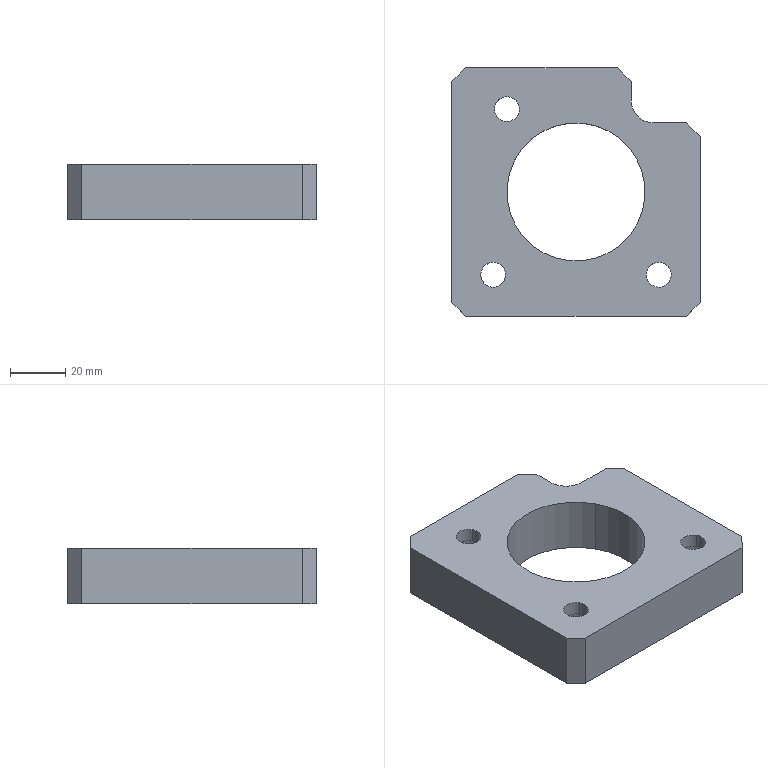Part | CATIA | 1 solid | 31 faces | box 90 x 90 x 20 mm | volume 102848 mm3 | plane 16 | cylinder 15 | commonest cylinder face diameters 9 x6 15 x6 50 x2 16 x1
STEP:
#1=CARTESIAN_POINT('',(500.,-120.,-5.5));
#2=VERTEX_POINT('',#1);
#3=CARTESIAN_POINT('',(500.,-120.,14.5));
#4=VERTEX_POINT('',#3);
#5=CARTESIAN_POINT('',(500.,-120.,4.5));
#6=DIRECTION('',(0.,0.,-1.));
#7=VECTOR('',#6,1.);
#8=LINE('',#5,#7);
#9=EDGE_CURVE('',#2,#4,#8,.F.);
#10=ORIENTED_EDGE('',*,*,#9,.F.);
#11=CARTESIAN_POINT('',(495.,-125.,-5.5));
#12=VERTEX_POINT('',#11);
#13=CARTESIAN_POINT('',(497.5,-122.5,-5.5));
#14=DIRECTION('',(0.7071,0.7071,0.));
#15=VECTOR('',#14,1.);
#16=LINE('',#13,#15);
#17=EDGE_CURVE('',#2,#12,#16,.F.);
#18=ORIENTED_EDGE('',*,*,#17,.T.);
#19=CARTESIAN_POINT('',(495.,-125.,14.5));
#20=VERTEX_POINT('',#19);
#21=CARTESIAN_POINT('',(495.,-125.,4.5));
#22=DIRECTION('',(0.,0.,-1.));
#23=VECTOR('',#22,1.);
#24=LINE('',#21,#23);
#25=EDGE_CURVE('',#12,#20,#24,.F.);
#26=ORIENTED_EDGE('',*,*,#25,.T.);
#27=CARTESIAN_POINT('',(497.5,-122.5,14.5));
#28=DIRECTION('',(0.7071,0.7071,0.));
#29=VECTOR('',#28,1.);
#30=LINE('',#27,#29);
#31=EDGE_CURVE('',#20,#4,#30,.T.);
#32=ORIENTED_EDGE('',*,*,#31,.T.);
#33=EDGE_LOOP('',(#10,#18,#26,#32));
#34=FACE_OUTER_BOUND('',#33,.T.);
#35=CARTESIAN_POINT('',(495.,-125.,18.5));
#36=DIRECTION('',(0.7071,-0.7071,0.));
#37=DIRECTION('',(0.,0.,-1.));
#38=AXIS2_PLACEMENT_3D('',#35,#36,#37);
#39=PLANE('',#38);
#40=ADVANCED_FACE('',(#34),#39,.F.);
#41=CARTESIAN_POINT('',(495.,-205.,-5.5));
#42=VERTEX_POINT('',#41);
#43=CARTESIAN_POINT('',(495.,-205.,14.5));
#44=VERTEX_POINT('',#43);
#45=CARTESIAN_POINT('',(495.,-205.,4.5));
#46=DIRECTION('',(0.,0.,1.));
#47=VECTOR('',#46,1.);
#48=LINE('',#45,#47);
#49=EDGE_CURVE('',#42,#44,#48,.T.);
#50=ORIENTED_EDGE('',*,*,#49,.T.);
#51=CARTESIAN_POINT('',(495.,-165.,14.5));
#52=DIRECTION('',(0.,1.,0.));
#53=VECTOR('',#52,1.);
#54=LINE('',#51,#53);
#55=EDGE_CURVE('',#20,#44,#54,.F.);
#56=ORIENTED_EDGE('',*,*,#55,.F.);
#57=ORIENTED_EDGE('',*,*,#25,.F.);
#58=CARTESIAN_POINT('',(495.,-165.,-5.5));
#59=DIRECTION('',(0.,1.,0.));
#60=VECTOR('',#59,1.);
#61=LINE('',#58,#60);
#62=EDGE_CURVE('',#12,#42,#61,.F.);
#63=ORIENTED_EDGE('',*,*,#62,.T.);
#64=EDGE_LOOP('',(#50,#56,#57,#63));
#65=FACE_OUTER_BOUND('',#64,.T.);
#66=CARTESIAN_POINT('',(495.,-210.,-5.5));
#67=DIRECTION('',(1.,0.,0.));
#68=DIRECTION('',(0.,1.,0.));
#69=AXIS2_PLACEMENT_3D('',#66,#67,#68);
#70=PLANE('',#69);
#71=ADVANCED_FACE('',(#65),#70,.F.);
#72=ORIENTED_EDGE('',*,*,#49,.F.);
#73=CARTESIAN_POINT('',(500.,-210.,-5.5));
#74=VERTEX_POINT('',#73);
#75=CARTESIAN_POINT('',(497.5,-207.5,-5.5));
#76=DIRECTION('',(0.7071,-0.7071,0.));
#77=VECTOR('',#76,1.);
#78=LINE('',#75,#77);
#79=EDGE_CURVE('',#42,#74,#78,.T.);
#80=ORIENTED_EDGE('',*,*,#79,.T.);
#81=CARTESIAN_POINT('',(500.,-210.,14.5));
#82=VERTEX_POINT('',#81);
#83=CARTESIAN_POINT('',(500.,-210.,4.5));
#84=DIRECTION('',(0.,0.,1.));
#85=VECTOR('',#84,1.);
#86=LINE('',#83,#85);
#87=EDGE_CURVE('',#74,#82,#86,.T.);
#88=ORIENTED_EDGE('',*,*,#87,.T.);
#89=CARTESIAN_POINT('',(497.5,-207.5,14.5));
#90=DIRECTION('',(0.7071,-0.7071,0.));
#91=VECTOR('',#90,1.);
#92=LINE('',#89,#91);
#93=EDGE_CURVE('',#82,#44,#92,.F.);
#94=ORIENTED_EDGE('',*,*,#93,.T.);
#95=EDGE_LOOP('',(#72,#80,#88,#94));
#96=FACE_OUTER_BOUND('',#95,.T.);
#97=CARTESIAN_POINT('',(495.,-205.,-9.5));
#98=DIRECTION('',(0.7071,0.7071,0.));
#99=DIRECTION('',(0.,0.,1.));
#100=AXIS2_PLACEMENT_3D('',#97,#98,#99);
#101=PLANE('',#100);
#102=ADVANCED_FACE('',(#96),#101,.F.);
#103=CARTESIAN_POINT('',(580.,-210.,-5.5));
#104=VERTEX_POINT('',#103);
#105=CARTESIAN_POINT('',(580.,-210.,14.5));
#106=VERTEX_POINT('',#105);
#107=CARTESIAN_POINT('',(580.,-210.,4.5));
#108=DIRECTION('',(0.,0.,-1.));
#109=VECTOR('',#108,1.);
#110=LINE('',#107,#109);
#111=EDGE_CURVE('',#104,#106,#110,.F.);
#112=ORIENTED_EDGE('',*,*,#111,.T.);
#113=CARTESIAN_POINT('',(540.,-210.,14.5));
#114=DIRECTION('',(-1.,0.,0.));
#115=VECTOR('',#114,1.);
#116=LINE('',#113,#115);
#117=EDGE_CURVE('',#82,#106,#116,.F.);
#118=ORIENTED_EDGE('',*,*,#117,.F.);
#119=ORIENTED_EDGE('',*,*,#87,.F.);
#120=CARTESIAN_POINT('',(540.,-210.,-5.5));
#121=DIRECTION('',(-1.,0.,0.));
#122=VECTOR('',#121,1.);
#123=LINE('',#120,#122);
#124=EDGE_CURVE('',#74,#104,#123,.F.);
#125=ORIENTED_EDGE('',*,*,#124,.T.);
#126=EDGE_LOOP('',(#112,#118,#119,#125));
#127=FACE_OUTER_BOUND('',#126,.T.);
#128=CARTESIAN_POINT('',(585.,-210.,-5.5));
#129=DIRECTION('',(0.,1.,0.));
#130=DIRECTION('',(-1.,0.,0.));
#131=AXIS2_PLACEMENT_3D('',#128,#129,#130);
#132=PLANE('',#131);
#133=ADVANCED_FACE('',(#127),#132,.F.);
#134=ORIENTED_EDGE('',*,*,#111,.F.);
#135=CARTESIAN_POINT('',(585.,-205.,-5.5));
#136=VERTEX_POINT('',#135);
#137=CARTESIAN_POINT('',(582.5,-207.5,-5.5));
#138=DIRECTION('',(-0.7071,-0.7071,0.));
#139=VECTOR('',#138,1.);
#140=LINE('',#137,#139);
#141=EDGE_CURVE('',#104,#136,#140,.F.);
#142=ORIENTED_EDGE('',*,*,#141,.T.);
#143=CARTESIAN_POINT('',(585.,-205.,14.5));
#144=VERTEX_POINT('',#143);
#145=CARTESIAN_POINT('',(585.,-205.,4.5));
#146=DIRECTION('',(0.,0.,-1.));
#147=VECTOR('',#146,1.);
#148=LINE('',#145,#147);
#149=EDGE_CURVE('',#136,#144,#148,.F.);
#150=ORIENTED_EDGE('',*,*,#149,.T.);
#151=CARTESIAN_POINT('',(582.5,-207.5,14.5));
#152=DIRECTION('',(-0.7071,-0.7071,0.));
#153=VECTOR('',#152,1.);
#154=LINE('',#151,#153);
#155=EDGE_CURVE('',#144,#106,#154,.T.);
#156=ORIENTED_EDGE('',*,*,#155,.T.);
#157=EDGE_LOOP('',(#134,#142,#150,#156));
#158=FACE_OUTER_BOUND('',#157,.T.);
#159=CARTESIAN_POINT('',(585.,-205.,18.5));
#160=DIRECTION('',(-0.7071,0.7071,0.));
#161=DIRECTION('',(0.,0.,-1.));
#162=AXIS2_PLACEMENT_3D('',#159,#160,#161);
#163=PLANE('',#162);
#164=ADVANCED_FACE('',(#158),#163,.F.);
#165=CARTESIAN_POINT('',(518.06,-176.986,14.5));
#166=VERTEX_POINT('',#165);
#167=CARTESIAN_POINT('',(561.94,-153.014,14.5));
#168=VERTEX_POINT('',#167);
#169=CARTESIAN_POINT('',(540.,-165.,14.5));
#170=DIRECTION('',(0.,0.,1.));
#171=AXIS2_PLACEMENT_3D('',#169,#170,$);
#172=CIRCLE('',#171,25.);
#173=EDGE_CURVE('',#166,#168,#172,.T.);
#174=ORIENTED_EDGE('',*,*,#173,.T.);
#175=CARTESIAN_POINT('',(561.94,-153.014,-5.5));
#176=VERTEX_POINT('',#175);
#177=CARTESIAN_POINT('',(561.94,-153.014,9.3));
#178=DIRECTION('',(0.,0.,1.));
#179=VECTOR('',#178,1.);
#180=LINE('',#177,#179);
#181=EDGE_CURVE('',#168,#176,#180,.F.);
#182=ORIENTED_EDGE('',*,*,#181,.T.);
#183=CARTESIAN_POINT('',(518.06,-176.986,-5.5));
#184=VERTEX_POINT('',#183);
#185=CARTESIAN_POINT('',(540.,-165.,-5.5));
#186=DIRECTION('',(0.,0.,1.));
#187=AXIS2_PLACEMENT_3D('',#185,#186,$);
#188=CIRCLE('',#187,25.);
#189=EDGE_CURVE('',#184,#176,#188,.T.);
#190=ORIENTED_EDGE('',*,*,#189,.F.);
#191=CARTESIAN_POINT('',(518.06,-176.986,9.3));
#192=DIRECTION('',(0.,0.,1.));
#193=VECTOR('',#192,1.);
#194=LINE('',#191,#193);
#195=EDGE_CURVE('',#166,#184,#194,.F.);
#196=ORIENTED_EDGE('',*,*,#195,.F.);
#197=EDGE_LOOP('',(#174,#182,#190,#196));
#198=FACE_OUTER_BOUND('',#197,.T.);
#199=CARTESIAN_POINT('',(540.,-165.,-5.4));
#200=DIRECTION('',(0.,0.,1.));
#201=DIRECTION('',(0.8776,0.4794,0.));
#202=AXIS2_PLACEMENT_3D('',#199,#200,#201);
#203=CYLINDRICAL_SURFACE('',#202,25.);
#204=ADVANCED_FACE('',(#198),#203,.F.);
#205=CARTESIAN_POINT('',(540.,-165.,14.5));
#206=DIRECTION('',(0.,0.,1.));
#207=AXIS2_PLACEMENT_3D('',#205,#206,$);
#208=CIRCLE('',#207,25.);
#209=EDGE_CURVE('',#168,#166,#208,.T.);
#210=ORIENTED_EDGE('',*,*,#209,.T.);
#211=ORIENTED_EDGE('',*,*,#195,.T.);
#212=CARTESIAN_POINT('',(540.,-165.,-5.5));
#213=DIRECTION('',(0.,0.,1.));
#214=AXIS2_PLACEMENT_3D('',#212,#213,$);
#215=CIRCLE('',#214,25.);
#216=EDGE_CURVE('',#176,#184,#215,.T.);
#217=ORIENTED_EDGE('',*,*,#216,.F.);
#218=ORIENTED_EDGE('',*,*,#181,.F.);
#219=EDGE_LOOP('',(#210,#211,#217,#218));
#220=FACE_OUTER_BOUND('',#219,.T.);
#221=ADVANCED_FACE('',(#220),#203,.F.);
#222=CARTESIAN_POINT('',(521.582,-131.404,9.5));
#223=VERTEX_POINT('',#222);
#224=CARTESIAN_POINT('',(508.418,-138.596,9.5));
#225=VERTEX_POINT('',#224);
#226=CARTESIAN_POINT('',(515.,-135.,9.5));
#227=DIRECTION('',(0.,0.,1.));
#228=AXIS2_PLACEMENT_3D('',#226,#227,$);
#229=CIRCLE('',#228,7.5);
#230=EDGE_CURVE('',#223,#225,#229,.T.);
#231=ORIENTED_EDGE('',*,*,#230,.F.);
#232=CARTESIAN_POINT('',(515.,-135.,9.5));
#233=DIRECTION('',(0.,0.,1.));
#234=AXIS2_PLACEMENT_3D('',#232,#233,$);
#235=CIRCLE('',#234,7.5);
#236=EDGE_CURVE('',#225,#223,#235,.T.);
#237=ORIENTED_EDGE('',*,*,#236,.F.);
#238=EDGE_LOOP('',(#231,#237));
#239=FACE_OUTER_BOUND('',#238,.T.);
#240=CARTESIAN_POINT('',(511.051,-137.157,9.5));
#241=VERTEX_POINT('',#240);
#242=CARTESIAN_POINT('',(518.949,-132.843,9.5));
#243=VERTEX_POINT('',#242);
#244=CARTESIAN_POINT('',(515.,-135.,9.5));
#245=DIRECTION('',(0.,0.,1.));
#246=AXIS2_PLACEMENT_3D('',#244,#245,$);
#247=CIRCLE('',#246,4.5);
#248=EDGE_CURVE('',#241,#243,#247,.T.);
#249=ORIENTED_EDGE('',*,*,#248,.T.);
#250=CARTESIAN_POINT('',(515.,-135.,9.5));
#251=DIRECTION('',(0.,0.,1.));
#252=AXIS2_PLACEMENT_3D('',#250,#251,$);
#253=CIRCLE('',#252,4.5);
#254=EDGE_CURVE('',#243,#241,#253,.T.);
#255=ORIENTED_EDGE('',*,*,#254,.T.);
#256=EDGE_LOOP('',(#249,#255));
#257=FACE_BOUND('',#256,.T.);
#258=CARTESIAN_POINT('',(574.5,-195.,9.5));
#259=DIRECTION('',(0.,0.,1.));
#260=DIRECTION('',(1.,0.,0.));
#261=AXIS2_PLACEMENT_3D('',#258,#259,#260);
#262=PLANE('',#261);
#263=ADVANCED_FACE('',(#239,#257),#262,.F.);
#264=CARTESIAN_POINT('',(508.418,-138.596,-5.5));
#265=VERTEX_POINT('',#264);
#266=CARTESIAN_POINT('',(521.582,-131.404,-5.5));
#267=VERTEX_POINT('',#266);
#268=CARTESIAN_POINT('',(515.,-135.,-5.5));
#269=DIRECTION('',(0.,0.,1.));
#270=AXIS2_PLACEMENT_3D('',#268,#269,$);
#271=CIRCLE('',#270,7.5);
#272=EDGE_CURVE('',#265,#267,#271,.T.);
#273=ORIENTED_EDGE('',*,*,#272,.F.);
#274=CARTESIAN_POINT('',(508.418,-138.596,1.8));
#275=DIRECTION('',(0.,0.,1.));
#276=VECTOR('',#275,1.);
#277=LINE('',#274,#276);
#278=EDGE_CURVE('',#225,#265,#277,.F.);
#279=ORIENTED_EDGE('',*,*,#278,.F.);
#280=ORIENTED_EDGE('',*,*,#236,.T.);
#281=CARTESIAN_POINT('',(521.582,-131.404,1.8));
#282=DIRECTION('',(0.,0.,1.));
#283=VECTOR('',#282,1.);
#284=LINE('',#281,#283);
#285=EDGE_CURVE('',#223,#267,#284,.F.);
#286=ORIENTED_EDGE('',*,*,#285,.T.);
#287=EDGE_LOOP('',(#273,#279,#280,#286));
#288=FACE_OUTER_BOUND('',#287,.T.);
#289=CARTESIAN_POINT('',(515.,-135.,-5.4));
#290=DIRECTION('',(0.,0.,1.));
#291=DIRECTION('',(0.8776,0.4794,0.));
#292=AXIS2_PLACEMENT_3D('',#289,#290,#291);
#293=CYLINDRICAL_SURFACE('',#292,7.5);
#294=ADVANCED_FACE('',(#288),#293,.F.);
#295=CARTESIAN_POINT('',(515.,-135.,-5.5));
#296=DIRECTION('',(0.,0.,1.));
#297=AXIS2_PLACEMENT_3D('',#295,#296,$);
#298=CIRCLE('',#297,7.5);
#299=EDGE_CURVE('',#267,#265,#298,.T.);
#300=ORIENTED_EDGE('',*,*,#299,.F.);
#301=ORIENTED_EDGE('',*,*,#285,.F.);
#302=ORIENTED_EDGE('',*,*,#230,.T.);
#303=ORIENTED_EDGE('',*,*,#278,.T.);
#304=EDGE_LOOP('',(#300,#301,#302,#303));
#305=FACE_OUTER_BOUND('',#304,.T.);
#306=ADVANCED_FACE('',(#305),#293,.F.);
#307=CARTESIAN_POINT('',(518.949,-132.843,14.5));
#308=VERTEX_POINT('',#307);
#309=CARTESIAN_POINT('',(511.051,-137.157,14.5));
#310=VERTEX_POINT('',#309);
#311=CARTESIAN_POINT('',(515.,-135.,14.5));
#312=DIRECTION('',(0.,0.,1.));
#313=AXIS2_PLACEMENT_3D('',#311,#312,$);
#314=CIRCLE('',#313,4.5);
#315=EDGE_CURVE('',#308,#310,#314,.T.);
#316=ORIENTED_EDGE('',*,*,#315,.T.);
#317=CARTESIAN_POINT('',(511.051,-137.157,12.2));
#318=DIRECTION('',(0.,0.,1.));
#319=VECTOR('',#318,1.);
#320=LINE('',#317,#319);
#321=EDGE_CURVE('',#310,#241,#320,.F.);
#322=ORIENTED_EDGE('',*,*,#321,.T.);
#323=ORIENTED_EDGE('',*,*,#254,.F.);
#324=CARTESIAN_POINT('',(518.949,-132.843,12.2));
#325=DIRECTION('',(0.,0.,1.));
#326=VECTOR('',#325,1.);
#327=LINE('',#324,#326);
#328=EDGE_CURVE('',#308,#243,#327,.F.);
#329=ORIENTED_EDGE('',*,*,#328,.F.);
#330=EDGE_LOOP('',(#316,#322,#323,#329));
#331=FACE_OUTER_BOUND('',#330,.T.);
#332=CARTESIAN_POINT('',(515.,-135.,-5.4));
#333=DIRECTION('',(0.,0.,1.));
#334=DIRECTION('',(0.8776,0.4794,0.));
#335=AXIS2_PLACEMENT_3D('',#332,#333,#334);
#336=CYLINDRICAL_SURFACE('',#335,4.5);
#337=ADVANCED_FACE('',(#331),#336,.F.);
#338=CARTESIAN_POINT('',(515.,-135.,14.5));
#339=DIRECTION('',(0.,0.,1.));
#340=AXIS2_PLACEMENT_3D('',#338,#339,$);
#341=CIRCLE('',#340,4.5);
#342=EDGE_CURVE('',#310,#308,#341,.T.);
#343=ORIENTED_EDGE('',*,*,#342,.T.);
#344=ORIENTED_EDGE('',*,*,#328,.T.);
#345=ORIENTED_EDGE('',*,*,#248,.F.);
#346=ORIENTED_EDGE('',*,*,#321,.F.);
#347=EDGE_LOOP('',(#343,#344,#345,#346));
#348=FACE_OUTER_BOUND('',#347,.T.);
#349=ADVANCED_FACE('',(#348),#336,.F.);
#350=CARTESIAN_POINT('',(516.582,-191.404,9.5));
#351=VERTEX_POINT('',#350);
#352=CARTESIAN_POINT('',(503.418,-198.596,9.5));
#353=VERTEX_POINT('',#352);
#354=CARTESIAN_POINT('',(510.,-195.,9.5));
#355=DIRECTION('',(0.,0.,1.));
#356=AXIS2_PLACEMENT_3D('',#354,#355,$);
#357=CIRCLE('',#356,7.5);
#358=EDGE_CURVE('',#351,#353,#357,.T.);
#359=ORIENTED_EDGE('',*,*,#358,.F.);
#360=CARTESIAN_POINT('',(510.,-195.,9.5));
#361=DIRECTION('',(0.,0.,1.));
#362=AXIS2_PLACEMENT_3D('',#360,#361,$);
#363=CIRCLE('',#362,7.5);
#364=EDGE_CURVE('',#353,#351,#363,.T.);
#365=ORIENTED_EDGE('',*,*,#364,.F.);
#366=EDGE_LOOP('',(#359,#365));
#367=FACE_OUTER_BOUND('',#366,.T.);
#368=CARTESIAN_POINT('',(506.051,-197.157,9.5));
#369=VERTEX_POINT('',#368);
#370=CARTESIAN_POINT('',(513.949,-192.843,9.5));
#371=VERTEX_POINT('',#370);
#372=CARTESIAN_POINT('',(510.,-195.,9.5));
#373=DIRECTION('',(0.,0.,1.));
#374=AXIS2_PLACEMENT_3D('',#372,#373,$);
#375=CIRCLE('',#374,4.5);
#376=EDGE_CURVE('',#369,#371,#375,.T.);
#377=ORIENTED_EDGE('',*,*,#376,.T.);
#378=CARTESIAN_POINT('',(510.,-195.,9.5));
#379=DIRECTION('',(0.,0.,1.));
#380=AXIS2_PLACEMENT_3D('',#378,#379,$);
#381=CIRCLE('',#380,4.5);
#382=EDGE_CURVE('',#371,#369,#381,.T.);
#383=ORIENTED_EDGE('',*,*,#382,.T.);
#384=EDGE_LOOP('',(#377,#383));
#385=FACE_BOUND('',#384,.T.);
#386=ADVANCED_FACE('',(#367,#385),#262,.F.);
#387=CARTESIAN_POINT('',(503.418,-198.596,-5.5));
#388=VERTEX_POINT('',#387);
#389=CARTESIAN_POINT('',(516.582,-191.404,-5.5));
#390=VERTEX_POINT('',#389);
#391=CARTESIAN_POINT('',(510.,-195.,-5.5));
#392=DIRECTION('',(0.,0.,1.));
#393=AXIS2_PLACEMENT_3D('',#391,#392,$);
#394=CIRCLE('',#393,7.5);
#395=EDGE_CURVE('',#388,#390,#394,.T.);
#396=ORIENTED_EDGE('',*,*,#395,.F.);
#397=CARTESIAN_POINT('',(503.418,-198.596,1.8));
#398=DIRECTION('',(0.,0.,1.));
#399=VECTOR('',#398,1.);
#400=LINE('',#397,#399);
#401=EDGE_CURVE('',#353,#388,#400,.F.);
#402=ORIENTED_EDGE('',*,*,#401,.F.);
#403=ORIENTED_EDGE('',*,*,#364,.T.);
#404=CARTESIAN_POINT('',(516.582,-191.404,1.8));
#405=DIRECTION('',(0.,0.,1.));
#406=VECTOR('',#405,1.);
#407=LINE('',#404,#406);
#408=EDGE_CURVE('',#351,#390,#407,.F.);
#409=ORIENTED_EDGE('',*,*,#408,.T.);
#410=EDGE_LOOP('',(#396,#402,#403,#409));
#411=FACE_OUTER_BOUND('',#410,.T.);
#412=CARTESIAN_POINT('',(510.,-195.,-5.4));
#413=DIRECTION('',(0.,0.,1.));
#414=DIRECTION('',(0.8776,0.4794,0.));
#415=AXIS2_PLACEMENT_3D('',#412,#413,#414);
#416=CYLINDRICAL_SURFACE('',#415,7.5);
#417=ADVANCED_FACE('',(#411),#416,.F.);
#418=CARTESIAN_POINT('',(510.,-195.,-5.5));
#419=DIRECTION('',(0.,0.,1.));
#420=AXIS2_PLACEMENT_3D('',#418,#419,$);
#421=CIRCLE('',#420,7.5);
#422=EDGE_CURVE('',#390,#388,#421,.T.);
#423=ORIENTED_EDGE('',*,*,#422,.F.);
#424=ORIENTED_EDGE('',*,*,#408,.F.);
#425=ORIENTED_EDGE('',*,*,#358,.T.);
#426=ORIENTED_EDGE('',*,*,#401,.T.);
#427=EDGE_LOOP('',(#423,#424,#425,#426));
#428=FACE_OUTER_BOUND('',#427,.T.);
#429=ADVANCED_FACE('',(#428),#416,.F.);
#430=CARTESIAN_POINT('',(513.949,-192.843,14.5));
#431=VERTEX_POINT('',#430);
#432=CARTESIAN_POINT('',(506.051,-197.157,14.5));
#433=VERTEX_POINT('',#432);
#434=CARTESIAN_POINT('',(510.,-195.,14.5));
#435=DIRECTION('',(0.,0.,1.));
#436=AXIS2_PLACEMENT_3D('',#434,#435,$);
#437=CIRCLE('',#436,4.5);
#438=EDGE_CURVE('',#431,#433,#437,.T.);
#439=ORIENTED_EDGE('',*,*,#438,.T.);
#440=CARTESIAN_POINT('',(506.051,-197.157,12.2));
#441=DIRECTION('',(0.,0.,1.));
#442=VECTOR('',#441,1.);
#443=LINE('',#440,#442);
#444=EDGE_CURVE('',#433,#369,#443,.F.);
#445=ORIENTED_EDGE('',*,*,#444,.T.);
#446=ORIENTED_EDGE('',*,*,#382,.F.);
#447=CARTESIAN_POINT('',(513.949,-192.843,12.2));
#448=DIRECTION('',(0.,0.,1.));
#449=VECTOR('',#448,1.);
#450=LINE('',#447,#449);
#451=EDGE_CURVE('',#431,#371,#450,.F.);
#452=ORIENTED_EDGE('',*,*,#451,.F.);
#453=EDGE_LOOP('',(#439,#445,#446,#452));
#454=FACE_OUTER_BOUND('',#453,.T.);
#455=CARTESIAN_POINT('',(510.,-195.,-5.4));
#456=DIRECTION('',(0.,0.,1.));
#457=DIRECTION('',(0.8776,0.4794,0.));
#458=AXIS2_PLACEMENT_3D('',#455,#456,#457);
#459=CYLINDRICAL_SURFACE('',#458,4.5);
#460=ADVANCED_FACE('',(#454),#459,.F.);
#461=CARTESIAN_POINT('',(510.,-195.,14.5));
#462=DIRECTION('',(0.,0.,1.));
#463=AXIS2_PLACEMENT_3D('',#461,#462,$);
#464=CIRCLE('',#463,4.5);
#465=EDGE_CURVE('',#433,#431,#464,.T.);
#466=ORIENTED_EDGE('',*,*,#465,.T.);
#467=ORIENTED_EDGE('',*,*,#451,.T.);
#468=ORIENTED_EDGE('',*,*,#376,.F.);
#469=ORIENTED_EDGE('',*,*,#444,.F.);
#470=EDGE_LOOP('',(#466,#467,#468,#469));
#471=FACE_OUTER_BOUND('',#470,.T.);
#472=ADVANCED_FACE('',(#471),#459,.F.);
#473=CARTESIAN_POINT('',(576.582,-191.404,9.5));
#474=VERTEX_POINT('',#473);
#475=CARTESIAN_POINT('',(563.418,-198.596,9.5));
#476=VERTEX_POINT('',#475);
#477=CARTESIAN_POINT('',(570.,-195.,9.5));
#478=DIRECTION('',(0.,0.,1.));
#479=AXIS2_PLACEMENT_3D('',#477,#478,$);
#480=CIRCLE('',#479,7.5);
#481=EDGE_CURVE('',#474,#476,#480,.T.);
#482=ORIENTED_EDGE('',*,*,#481,.F.);
#483=CARTESIAN_POINT('',(570.,-195.,9.5));
#484=DIRECTION('',(0.,0.,1.));
#485=AXIS2_PLACEMENT_3D('',#483,#484,$);
#486=CIRCLE('',#485,7.5);
#487=EDGE_CURVE('',#476,#474,#486,.T.);
#488=ORIENTED_EDGE('',*,*,#487,.F.);
#489=EDGE_LOOP('',(#482,#488));
#490=FACE_OUTER_BOUND('',#489,.T.);
#491=CARTESIAN_POINT('',(566.051,-197.157,9.5));
#492=VERTEX_POINT('',#491);
#493=CARTESIAN_POINT('',(573.949,-192.843,9.5));
#494=VERTEX_POINT('',#493);
#495=CARTESIAN_POINT('',(570.,-195.,9.5));
#496=DIRECTION('',(0.,0.,1.));
#497=AXIS2_PLACEMENT_3D('',#495,#496,$);
#498=CIRCLE('',#497,4.5);
#499=EDGE_CURVE('',#492,#494,#498,.T.);
#500=ORIENTED_EDGE('',*,*,#499,.T.);
#501=CARTESIAN_POINT('',(570.,-195.,9.5));
#502=DIRECTION('',(0.,0.,1.));
#503=AXIS2_PLACEMENT_3D('',#501,#502,$);
#504=CIRCLE('',#503,4.5);
#505=EDGE_CURVE('',#494,#492,#504,.T.);
#506=ORIENTED_EDGE('',*,*,#505,.T.);
#507=EDGE_LOOP('',(#500,#506));
#508=FACE_BOUND('',#507,.T.);
#509=ADVANCED_FACE('',(#490,#508),#262,.F.);
#510=CARTESIAN_POINT('',(563.418,-198.596,-5.5));
#511=VERTEX_POINT('',#510);
#512=CARTESIAN_POINT('',(576.582,-191.404,-5.5));
#513=VERTEX_POINT('',#512);
#514=CARTESIAN_POINT('',(570.,-195.,-5.5));
#515=DIRECTION('',(0.,0.,1.));
#516=AXIS2_PLACEMENT_3D('',#514,#515,$);
#517=CIRCLE('',#516,7.5);
#518=EDGE_CURVE('',#511,#513,#517,.T.);
#519=ORIENTED_EDGE('',*,*,#518,.F.);
#520=CARTESIAN_POINT('',(563.418,-198.596,1.8));
#521=DIRECTION('',(0.,0.,1.));
#522=VECTOR('',#521,1.);
#523=LINE('',#520,#522);
#524=EDGE_CURVE('',#476,#511,#523,.F.);
#525=ORIENTED_EDGE('',*,*,#524,.F.);
#526=ORIENTED_EDGE('',*,*,#487,.T.);
#527=CARTESIAN_POINT('',(576.582,-191.404,1.8));
#528=DIRECTION('',(0.,0.,1.));
#529=VECTOR('',#528,1.);
#530=LINE('',#527,#529);
#531=EDGE_CURVE('',#474,#513,#530,.F.);
#532=ORIENTED_EDGE('',*,*,#531,.T.);
#533=EDGE_LOOP('',(#519,#525,#526,#532));
#534=FACE_OUTER_BOUND('',#533,.T.);
#535=CARTESIAN_POINT('',(570.,-195.,-5.4));
#536=DIRECTION('',(0.,0.,1.));
#537=DIRECTION('',(0.8776,0.4794,0.));
#538=AXIS2_PLACEMENT_3D('',#535,#536,#537);
#539=CYLINDRICAL_SURFACE('',#538,7.5);
#540=ADVANCED_FACE('',(#534),#539,.F.);
#541=CARTESIAN_POINT('',(570.,-195.,-5.5));
#542=DIRECTION('',(0.,0.,1.));
#543=AXIS2_PLACEMENT_3D('',#541,#542,$);
#544=CIRCLE('',#543,7.5);
#545=EDGE_CURVE('',#513,#511,#544,.T.);
#546=ORIENTED_EDGE('',*,*,#545,.F.);
#547=ORIENTED_EDGE('',*,*,#531,.F.);
#548=ORIENTED_EDGE('',*,*,#481,.T.);
#549=ORIENTED_EDGE('',*,*,#524,.T.);
#550=EDGE_LOOP('',(#546,#547,#548,#549));
#551=FACE_OUTER_BOUND('',#550,.T.);
#552=ADVANCED_FACE('',(#551),#539,.F.);
#553=CARTESIAN_POINT('',(573.949,-192.843,14.5));
#554=VERTEX_POINT('',#553);
#555=CARTESIAN_POINT('',(566.051,-197.157,14.5));
#556=VERTEX_POINT('',#555);
#557=CARTESIAN_POINT('',(570.,-195.,14.5));
#558=DIRECTION('',(0.,0.,1.));
#559=AXIS2_PLACEMENT_3D('',#557,#558,$);
#560=CIRCLE('',#559,4.5);
#561=EDGE_CURVE('',#554,#556,#560,.T.);
#562=ORIENTED_EDGE('',*,*,#561,.T.);
#563=CARTESIAN_POINT('',(566.051,-197.157,12.2));
#564=DIRECTION('',(0.,0.,1.));
#565=VECTOR('',#564,1.);
#566=LINE('',#563,#565);
#567=EDGE_CURVE('',#556,#492,#566,.F.);
#568=ORIENTED_EDGE('',*,*,#567,.T.);
#569=ORIENTED_EDGE('',*,*,#505,.F.);
#570=CARTESIAN_POINT('',(573.949,-192.843,12.2));
#571=DIRECTION('',(0.,0.,1.));
#572=VECTOR('',#571,1.);
#573=LINE('',#570,#572);
#574=EDGE_CURVE('',#554,#494,#573,.F.);
#575=ORIENTED_EDGE('',*,*,#574,.F.);
#576=EDGE_LOOP('',(#562,#568,#569,#575));
#577=FACE_OUTER_BOUND('',#576,.T.);
#578=CARTESIAN_POINT('',(570.,-195.,-5.4));
#579=DIRECTION('',(0.,0.,1.));
#580=DIRECTION('',(0.8776,0.4794,0.));
#581=AXIS2_PLACEMENT_3D('',#578,#579,#580);
#582=CYLINDRICAL_SURFACE('',#581,4.5);
#583=ADVANCED_FACE('',(#577),#582,.F.);
#584=CARTESIAN_POINT('',(570.,-195.,14.5));
#585=DIRECTION('',(0.,0.,1.));
#586=AXIS2_PLACEMENT_3D('',#584,#585,$);
#587=CIRCLE('',#586,4.5);
#588=EDGE_CURVE('',#556,#554,#587,.T.);
#589=ORIENTED_EDGE('',*,*,#588,.T.);
#590=ORIENTED_EDGE('',*,*,#574,.T.);
#591=ORIENTED_EDGE('',*,*,#499,.F.);
#592=ORIENTED_EDGE('',*,*,#567,.F.);
#593=EDGE_LOOP('',(#589,#590,#591,#592));
#594=FACE_OUTER_BOUND('',#593,.T.);
#595=ADVANCED_FACE('',(#594),#582,.F.);
#596=CARTESIAN_POINT('',(560.,-132.,14.5));
#597=VERTEX_POINT('',#596);
#598=CARTESIAN_POINT('',(568.,-140.,14.5));
#599=VERTEX_POINT('',#598);
#600=CARTESIAN_POINT('',(568.,-132.,14.5));
#601=DIRECTION('',(0.,0.,-1.));
#602=AXIS2_PLACEMENT_3D('',#600,#601,$);
#603=CIRCLE('',#602,8.);
#604=EDGE_CURVE('',#597,#599,#603,.F.);
#605=ORIENTED_EDGE('',*,*,#604,.T.);
#606=CARTESIAN_POINT('',(568.,-140.,-5.5));
#607=VERTEX_POINT('',#606);
#608=CARTESIAN_POINT('',(568.,-140.,9.5));
#609=DIRECTION('',(0.,0.,-1.));
#610=VECTOR('',#609,1.);
#611=LINE('',#608,#610);
#612=EDGE_CURVE('',#607,#599,#611,.F.);
#613=ORIENTED_EDGE('',*,*,#612,.F.);
#614=CARTESIAN_POINT('',(560.,-132.,-5.5));
#615=VERTEX_POINT('',#614);
#616=CARTESIAN_POINT('',(568.,-132.,-5.5));
#617=DIRECTION('',(0.,0.,-1.));
#618=AXIS2_PLACEMENT_3D('',#616,#617,$);
#619=CIRCLE('',#618,8.);
#620=EDGE_CURVE('',#607,#615,#619,.T.);
#621=ORIENTED_EDGE('',*,*,#620,.T.);
#622=CARTESIAN_POINT('',(560.,-132.,9.5));
#623=DIRECTION('',(0.,0.,-1.));
#624=VECTOR('',#623,1.);
#625=LINE('',#622,#624);
#626=EDGE_CURVE('',#615,#597,#625,.F.);
#627=ORIENTED_EDGE('',*,*,#626,.T.);
#628=EDGE_LOOP('',(#605,#613,#621,#627));
#629=FACE_OUTER_BOUND('',#628,.T.);
#630=CARTESIAN_POINT('',(568.,-132.,9.5));
#631=DIRECTION('',(0.,0.,-1.));
#632=DIRECTION('',(0.,-1.,0.));
#633=AXIS2_PLACEMENT_3D('',#630,#631,#632);
#634=CYLINDRICAL_SURFACE('',#633,8.);
#635=ADVANCED_FACE('',(#629),#634,.F.);
#636=CARTESIAN_POINT('',(585.,-145.,-5.5));
#637=VERTEX_POINT('',#636);
#638=CARTESIAN_POINT('',(585.,-145.,14.5));
#639=VERTEX_POINT('',#638);
#640=CARTESIAN_POINT('',(585.,-145.,4.5));
#641=DIRECTION('',(0.,0.,-1.));
#642=VECTOR('',#641,1.);
#643=LINE('',#640,#642);
#644=EDGE_CURVE('',#637,#639,#643,.F.);
#645=ORIENTED_EDGE('',*,*,#644,.T.);
#646=CARTESIAN_POINT('',(585.,-175.,14.5));
#647=DIRECTION('',(0.,-1.,0.));
#648=VECTOR('',#647,1.);
#649=LINE('',#646,#648);
#650=EDGE_CURVE('',#144,#639,#649,.F.);
#651=ORIENTED_EDGE('',*,*,#650,.F.);
#652=ORIENTED_EDGE('',*,*,#149,.F.);
#653=CARTESIAN_POINT('',(585.,-175.,-5.5));
#654=DIRECTION('',(0.,-1.,0.));
#655=VECTOR('',#654,1.);
#656=LINE('',#653,#655);
#657=EDGE_CURVE('',#136,#637,#656,.F.);
#658=ORIENTED_EDGE('',*,*,#657,.T.);
#659=EDGE_LOOP('',(#645,#651,#652,#658));
#660=FACE_OUTER_BOUND('',#659,.T.);
#661=CARTESIAN_POINT('',(585.,-120.,-5.5));
#662=DIRECTION('',(-1.,0.,0.));
#663=DIRECTION('',(0.,-1.,0.));
#664=AXIS2_PLACEMENT_3D('',#661,#662,#663);
#665=PLANE('',#664);
#666=ADVANCED_FACE('',(#660),#665,.F.);
#667=CARTESIAN_POINT('',(580.,-140.,-5.5));
#668=VERTEX_POINT('',#667);
#669=CARTESIAN_POINT('',(580.,-140.,14.5));
#670=VERTEX_POINT('',#669);
#671=CARTESIAN_POINT('',(580.,-140.,4.5));
#672=DIRECTION('',(0.,0.,-1.));
#673=VECTOR('',#672,1.);
#674=LINE('',#671,#673);
#675=EDGE_CURVE('',#668,#670,#674,.F.);
#676=ORIENTED_EDGE('',*,*,#675,.F.);
#677=CARTESIAN_POINT('',(574.,-140.,-5.5));
#678=DIRECTION('',(1.,0.,0.));
#679=VECTOR('',#678,1.);
#680=LINE('',#677,#679);
#681=EDGE_CURVE('',#668,#607,#680,.F.);
#682=ORIENTED_EDGE('',*,*,#681,.T.);
#683=ORIENTED_EDGE('',*,*,#612,.T.);
#684=CARTESIAN_POINT('',(574.,-140.,14.5));
#685=DIRECTION('',(1.,0.,0.));
#686=VECTOR('',#685,1.);
#687=LINE('',#684,#686);
#688=EDGE_CURVE('',#599,#670,#687,.T.);
#689=ORIENTED_EDGE('',*,*,#688,.T.);
#690=EDGE_LOOP('',(#676,#682,#683,#689));
#691=FACE_OUTER_BOUND('',#690,.T.);
#692=CARTESIAN_POINT('',(568.,-140.,-5.5));
#693=DIRECTION('',(0.,-1.,0.));
#694=DIRECTION('',(1.,0.,0.));
#695=AXIS2_PLACEMENT_3D('',#692,#693,#694);
#696=PLANE('',#695);
#697=ADVANCED_FACE('',(#691),#696,.F.);
#698=ORIENTED_EDGE('',*,*,#644,.F.);
#699=CARTESIAN_POINT('',(582.5,-142.5,-5.5));
#700=DIRECTION('',(0.7071,-0.7071,0.));
#701=VECTOR('',#700,1.);
#702=LINE('',#699,#701);
#703=EDGE_CURVE('',#637,#668,#702,.F.);
#704=ORIENTED_EDGE('',*,*,#703,.T.);
#705=ORIENTED_EDGE('',*,*,#675,.T.);
#706=CARTESIAN_POINT('',(582.5,-142.5,14.5));
#707=DIRECTION('',(0.7071,-0.7071,0.));
#708=VECTOR('',#707,1.);
#709=LINE('',#706,#708);
#710=EDGE_CURVE('',#670,#639,#709,.T.);
#711=ORIENTED_EDGE('',*,*,#710,.T.);
#712=EDGE_LOOP('',(#698,#704,#705,#711));
#713=FACE_OUTER_BOUND('',#712,.T.);
#714=CARTESIAN_POINT('',(580.,-140.,18.5));
#715=DIRECTION('',(-0.7071,-0.7071,0.));
#716=DIRECTION('',(0.,0.,-1.));
#717=AXIS2_PLACEMENT_3D('',#714,#715,#716);
#718=PLANE('',#717);
#719=ADVANCED_FACE('',(#713),#718,.F.);
#720=CARTESIAN_POINT('',(555.,-120.,-5.5));
#721=VERTEX_POINT('',#720);
#722=CARTESIAN_POINT('',(555.,-120.,14.5));
#723=VERTEX_POINT('',#722);
#724=CARTESIAN_POINT('',(555.,-120.,4.5));
#725=DIRECTION('',(0.,0.,1.));
#726=VECTOR('',#725,1.);
#727=LINE('',#724,#726);
#728=EDGE_CURVE('',#721,#723,#727,.T.);
#729=ORIENTED_EDGE('',*,*,#728,.F.);
#730=CARTESIAN_POINT('',(527.5,-120.,-5.5));
#731=DIRECTION('',(1.,0.,0.));
#732=VECTOR('',#731,1.);
#733=LINE('',#730,#732);
#734=EDGE_CURVE('',#721,#2,#733,.F.);
#735=ORIENTED_EDGE('',*,*,#734,.T.);
#736=ORIENTED_EDGE('',*,*,#9,.T.);
#737=CARTESIAN_POINT('',(527.5,-120.,14.5));
#738=DIRECTION('',(1.,0.,0.));
#739=VECTOR('',#738,1.);
#740=LINE('',#737,#739);
#741=EDGE_CURVE('',#723,#4,#740,.F.);
#742=ORIENTED_EDGE('',*,*,#741,.F.);
#743=EDGE_LOOP('',(#729,#735,#736,#742));
#744=FACE_OUTER_BOUND('',#743,.T.);
#745=CARTESIAN_POINT('',(495.,-120.,-5.5));
#746=DIRECTION('',(0.,-1.,0.));
#747=DIRECTION('',(1.,0.,0.));
#748=AXIS2_PLACEMENT_3D('',#745,#746,#747);
#749=PLANE('',#748);
#750=ADVANCED_FACE('',(#744),#749,.F.);
#751=CARTESIAN_POINT('',(560.,-125.,14.5));
#752=VERTEX_POINT('',#751);
#753=CARTESIAN_POINT('',(560.,-128.5,14.5));
#754=DIRECTION('',(0.,1.,0.));
#755=VECTOR('',#754,1.);
#756=LINE('',#753,#755);
#757=EDGE_CURVE('',#597,#752,#756,.T.);
#758=ORIENTED_EDGE('',*,*,#757,.F.);
#759=ORIENTED_EDGE('',*,*,#626,.F.);
#760=CARTESIAN_POINT('',(560.,-125.,-5.5));
#761=VERTEX_POINT('',#760);
#762=CARTESIAN_POINT('',(560.,-128.5,-5.5));
#763=DIRECTION('',(0.,1.,0.));
#764=VECTOR('',#763,1.);
#765=LINE('',#762,#764);
#766=EDGE_CURVE('',#615,#761,#765,.T.);
#767=ORIENTED_EDGE('',*,*,#766,.T.);
#768=CARTESIAN_POINT('',(560.,-125.,4.5));
#769=DIRECTION('',(0.,0.,1.));
#770=VECTOR('',#769,1.);
#771=LINE('',#768,#770);
#772=EDGE_CURVE('',#761,#752,#771,.T.);
#773=ORIENTED_EDGE('',*,*,#772,.T.);
#774=EDGE_LOOP('',(#758,#759,#767,#773));
#775=FACE_OUTER_BOUND('',#774,.T.);
#776=CARTESIAN_POINT('',(560.,-132.,-5.5));
#777=DIRECTION('',(1.,0.,0.));
#778=DIRECTION('',(0.,1.,0.));
#779=AXIS2_PLACEMENT_3D('',#776,#777,#778);
#780=PLANE('',#779);
#781=ADVANCED_FACE('',(#775),#780,.T.);
#782=ORIENTED_EDGE('',*,*,#741,.T.);
#783=ORIENTED_EDGE('',*,*,#31,.F.);
#784=ORIENTED_EDGE('',*,*,#55,.T.);
#785=ORIENTED_EDGE('',*,*,#93,.F.);
#786=ORIENTED_EDGE('',*,*,#117,.T.);
#787=ORIENTED_EDGE('',*,*,#155,.F.);
#788=ORIENTED_EDGE('',*,*,#650,.T.);
#789=ORIENTED_EDGE('',*,*,#710,.F.);
#790=ORIENTED_EDGE('',*,*,#688,.F.);
#791=ORIENTED_EDGE('',*,*,#604,.F.);
#792=ORIENTED_EDGE('',*,*,#757,.T.);
#793=CARTESIAN_POINT('',(557.5,-122.5,14.5));
#794=DIRECTION('',(0.7071,-0.7071,0.));
#795=VECTOR('',#794,1.);
#796=LINE('',#793,#795);
#797=EDGE_CURVE('',#723,#752,#796,.T.);
#798=ORIENTED_EDGE('',*,*,#797,.F.);
#799=EDGE_LOOP('',(#782,#783,#784,#785,#786,#787,#788,#789,#790,#791,#792,#798));
#800=FACE_OUTER_BOUND('',#799,.T.);
#801=ORIENTED_EDGE('',*,*,#209,.F.);
#802=ORIENTED_EDGE('',*,*,#173,.F.);
#803=EDGE_LOOP('',(#801,#802));
#804=FACE_BOUND('',#803,.T.);
#805=ORIENTED_EDGE('',*,*,#588,.F.);
#806=ORIENTED_EDGE('',*,*,#561,.F.);
#807=EDGE_LOOP('',(#805,#806));
#808=FACE_BOUND('',#807,.T.);
#809=ORIENTED_EDGE('',*,*,#465,.F.);
#810=ORIENTED_EDGE('',*,*,#438,.F.);
#811=EDGE_LOOP('',(#809,#810));
#812=FACE_BOUND('',#811,.T.);
#813=ORIENTED_EDGE('',*,*,#342,.F.);
#814=ORIENTED_EDGE('',*,*,#315,.F.);
#815=EDGE_LOOP('',(#813,#814));
#816=FACE_BOUND('',#815,.T.);
#817=CARTESIAN_POINT('',(0.,0.,14.5));
#818=DIRECTION('',(0.,0.,1.));
#819=DIRECTION('',(1.,0.,0.));
#820=AXIS2_PLACEMENT_3D('',#817,#818,#819);
#821=PLANE('',#820);
#822=ADVANCED_FACE('',(#800,#804,#808,#812,#816),#821,.T.);
#823=CARTESIAN_POINT('',(557.5,-122.5,-5.5));
#824=DIRECTION('',(0.7071,-0.7071,0.));
#825=VECTOR('',#824,1.);
#826=LINE('',#823,#825);
#827=EDGE_CURVE('',#761,#721,#826,.F.);
#828=ORIENTED_EDGE('',*,*,#827,.F.);
#829=ORIENTED_EDGE('',*,*,#766,.F.);
#830=ORIENTED_EDGE('',*,*,#620,.F.);
#831=ORIENTED_EDGE('',*,*,#681,.F.);
#832=ORIENTED_EDGE('',*,*,#703,.F.);
#833=ORIENTED_EDGE('',*,*,#657,.F.);
#834=ORIENTED_EDGE('',*,*,#141,.F.);
#835=ORIENTED_EDGE('',*,*,#124,.F.);
#836=ORIENTED_EDGE('',*,*,#79,.F.);
#837=ORIENTED_EDGE('',*,*,#62,.F.);
#838=ORIENTED_EDGE('',*,*,#17,.F.);
#839=ORIENTED_EDGE('',*,*,#734,.F.);
#840=EDGE_LOOP('',(#828,#829,#830,#831,#832,#833,#834,#835,#836,#837,#838,#839));
#841=FACE_OUTER_BOUND('',#840,.T.);
#842=ORIENTED_EDGE('',*,*,#216,.T.);
#843=ORIENTED_EDGE('',*,*,#189,.T.);
#844=EDGE_LOOP('',(#842,#843));
#845=FACE_BOUND('',#844,.T.);
#846=ORIENTED_EDGE('',*,*,#545,.T.);
#847=ORIENTED_EDGE('',*,*,#518,.T.);
#848=EDGE_LOOP('',(#846,#847));
#849=FACE_BOUND('',#848,.T.);
#850=ORIENTED_EDGE('',*,*,#422,.T.);
#851=ORIENTED_EDGE('',*,*,#395,.T.);
#852=EDGE_LOOP('',(#850,#851));
#853=FACE_BOUND('',#852,.T.);
#854=ORIENTED_EDGE('',*,*,#299,.T.);
#855=ORIENTED_EDGE('',*,*,#272,.T.);
#856=EDGE_LOOP('',(#854,#855));
#857=FACE_BOUND('',#856,.T.);
#858=CARTESIAN_POINT('',(0.,0.,-5.5));
#859=DIRECTION('',(0.,0.,1.));
#860=DIRECTION('',(1.,0.,0.));
#861=AXIS2_PLACEMENT_3D('',#858,#859,#860);
#862=PLANE('',#861);
#863=ADVANCED_FACE('',(#841,#845,#849,#853,#857),#862,.F.);
#864=ORIENTED_EDGE('',*,*,#797,.T.);
#865=ORIENTED_EDGE('',*,*,#772,.F.);
#866=ORIENTED_EDGE('',*,*,#827,.T.);
#867=ORIENTED_EDGE('',*,*,#728,.T.);
#868=EDGE_LOOP('',(#864,#865,#866,#867));
#869=FACE_OUTER_BOUND('',#868,.T.);
#870=CARTESIAN_POINT('',(555.,-120.,-9.5));
#871=DIRECTION('',(0.7071,0.7071,0.));
#872=DIRECTION('',(0.,0.,1.));
#873=AXIS2_PLACEMENT_3D('',#870,#871,#872);
#874=PLANE('',#873);
#875=ADVANCED_FACE('',(#869),#874,.T.);
#876=CLOSED_SHELL('',(#40,#71,#102,#133,#164,#204,#221,#263,#294,#306,#337,#349,#386,#417,#429,#460,#472,#509,#540,#552,#583,#595,#635,#666,#697,#719,#750,#781,#822,#863,#875));
#877=MANIFOLD_SOLID_BREP('',#876);
#878=(LENGTH_UNIT()NAMED_UNIT(*)SI_UNIT(.MILLI.,.METRE.));
#879=UNCERTAINTY_MEASURE_WITH_UNIT(LENGTH_MEASURE(0.005),#878,'','');
#880=(NAMED_UNIT(*)PLANE_ANGLE_UNIT()SI_UNIT($,.RADIAN.));
#881=(NAMED_UNIT(*)SI_UNIT($,.STERADIAN.)SOLID_ANGLE_UNIT());
#882=(GEOMETRIC_REPRESENTATION_CONTEXT(3)GLOBAL_UNCERTAINTY_ASSIGNED_CONTEXT((#879))GLOBAL_UNIT_ASSIGNED_CONTEXT((#878,#880,#881))REPRESENTATION_CONTEXT('',''));
#883=ADVANCED_BREP_SHAPE_REPRESENTATION('',(#877),#882);